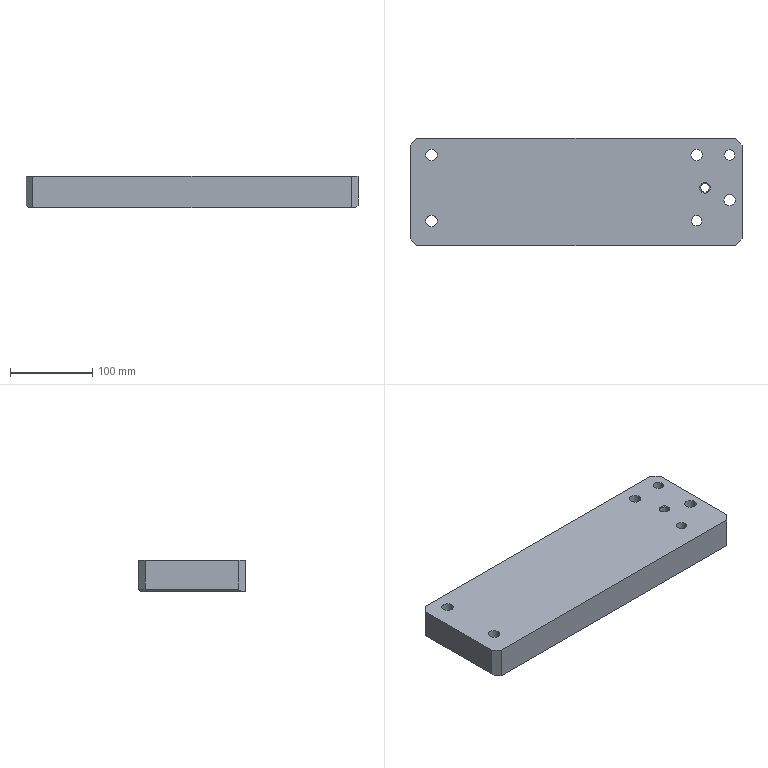Part | STEP file | 1_id650_x_t | 1 solid | 52 faces | box 403 x 130 x 38.1 mm | volume 1939605 mm3 | cylinder 28 | plane 22 | cone 2 | commonest cylinder face diameters 14 x14 20 x8 12.7 x4 10.716 x2